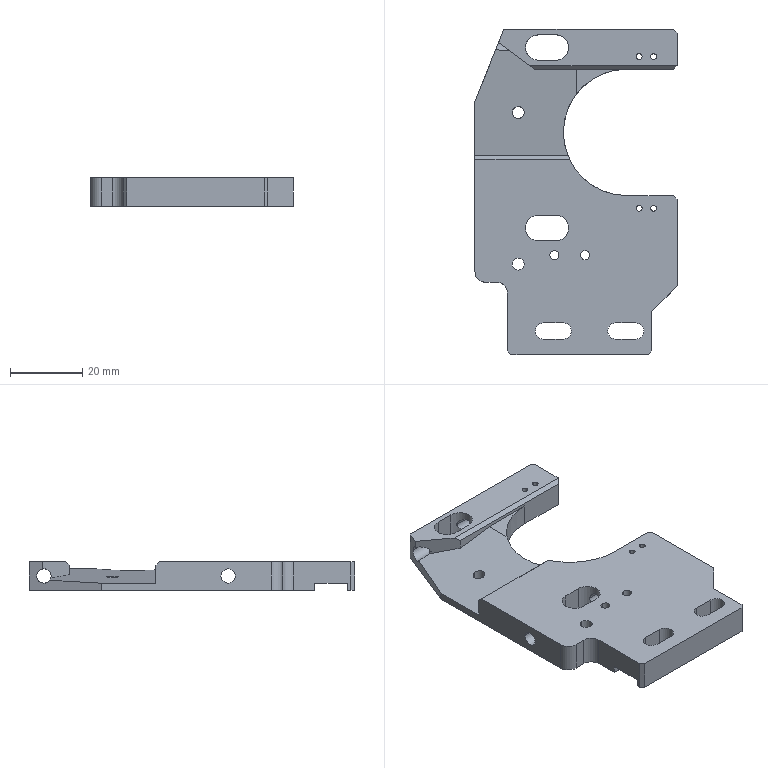NC program | NX | posted with a generic post | part box 56 x 90 x 8 mm
Whole program, first 1388 of 1533 lines:
N10 G17 G21 G94 G90
(ZLEVEL_PROFILE , TOOL : D10JING)
N12 T14 M6
N14 G54
N16 G17 G0 G90 X51.809 Y28.622 S7500 M3
N18 G43 Z30. H14
N20 Z-7.
N22 G94 G1 Z-8. F1000.
N24 X50.5 Y27.866
N26 G3 X50. Y27. R1.
N28 G1 Y-20.
N30 G2 X46.857 Y-24.642 R5.
N32 G1 X26.857 Y-32.642
N34 G2 X25. Y-33. R5.
N36 G1 X-22.
N38 G2 X-30. Y-25. R8.
N40 G1 Y-24.
N42 X-44.
N44 G2 X-47.536 Y-22.536 R5.
N46 G1 X-48.536 Y-21.536
N48 G2 X-50. Y-18. R5.
N50 G1 Y20.
N52 G2 X-48.536 Y23.536 R5.
N54 G1 X-47.536 Y24.536
N56 G2 X-44. Y26. R5.
N58 G1 X-35.071
N60 X-29.536 Y31.536
N62 G2 X-26. Y33. R5.
N64 G1 X-2.
N66 G2 X1.536 Y31.536 R5.
N68 G1 X2.536 Y30.536
N70 G2 X4. Y27. R5.
N72 G1 Y14.
N74 G3 X16.5 Y1.5 R12.5
N76 X29. Y14. R12.5
N78 G1 Y27.
N80 G2 X30.464 Y30.536 R5.
N82 G1 X31.464 Y31.536
N84 G2 X35. Y33. R5.
N86 G1 X44.
N88 G2 X47.536 Y31.536 R5.
N90 G1 X48.536 Y30.536
N92 G2 X50. Y27. R5.
N94 G3 X50.5 Y26.134 R1.
N96 G1 X52. Y25.268
N98 Z-7.
N100 G0 Z30.
N102 M5
(ZLEVEL_PROFILE_1 , TOOL : D4)
N104 T17 M6
N106 G54
N108 G17 G0 G90 X-8.5 Y-7.694 S7500 M3
N110 G43 Z30. H17
N112 Z1.5
N114 G94 G1 Y-5.199 Z1.369 F1000.
N116 X-8.75 Y-4.617 Z1.336
N118 X-9.214 Y-4.187 Z1.303
N120 X-9.782 Y-3.986 Z1.271
N122 X-10.542 Y-4.069 Z1.231
N124 X-11.167 Y-4.51 Z1.191
N126 X-11.5 Y-5.199 Z1.151
N128 Y-10.801 Z0.857
N130 X-11.17 Y-11.486 Z0.818
N132 X-10.55 Y-11.928 Z0.778
N134 X-9.795 Y-12.016 Z0.738
N136 X-9.225 Y-11.819 Z0.706
N138 X-8.754 Y-11.388 Z0.673
N140 X-8.5 Y-10.801 Z0.639
N142 Y-5.199 Z0.346
N144 X-8.75 Y-4.617 Z0.313
N146 X-9.214 Y-4.187 Z0.279
N148 X-9.782 Y-3.986 Z0.248
N150 X-10.542 Y-4.069 Z0.208
N152 X-11.167 Y-4.51 Z0.168
N154 X-11.5 Y-5.199 Z0.128
N156 Y-10.801 Z-0.166
N158 X-11.17 Y-11.486 Z-0.206
N160 X-10.55 Y-11.928 Z-0.246
N162 X-9.795 Y-12.016 Z-0.286
N164 X-9.225 Y-11.819 Z-0.317
N166 X-8.754 Y-11.388 Z-0.351
N168 X-8.5 Y-10.801 Z-0.384
N170 Y-10.5 Z-0.4
N172 Y-5.5 F1500.
N174 G3 X-10. Y-4. R1.5
N176 X-11.5 Y-5.5 R1.5
N178 G1 Y-10.5
N180 G3 X-10. Y-12. R1.5
N182 X-8.5 Y-10.5 R1.5
N184 G1 Y-5.644 Z-0.533
N186 X-8.539 Y-5.161 Z-0.547
N188 X-8.722 Y-4.714 Z-0.56
N190 X-8.899 Y-4.481 Z-0.568
N192 X-9.057 Y-4.37 Z-0.573
N194 X-9.375 Y-4.165 Z-0.584
N196 X-9.465 Y-4.129 Z-0.587
N198 X-9.773 Y-4.045 Z-0.596
N200 X-9.929 Y-4.024 Z-0.6
N202 X-10.209 Y-4.044 Z-0.608
N204 X-10.403 Y-4.075 Z-0.613
N206 X-10.63 Y-4.167 Z-0.62
N208 X-10.832 Y-4.283 Z-0.627
N210 X-11.045 Y-4.446 Z-0.634
N212 X-11.088 Y-4.501 Z-0.636
N214 X-11.174 Y-4.612 Z-0.64
N216 X-11.336 Y-4.881 Z-0.649
N218 X-11.399 Y-5.031 Z-0.653
N220 X-11.447 Y-5.213 Z-0.659
N222 X-11.483 Y-5.5 Z-0.667
N224 X-11.5 Y-5.743 Z-0.673
N226 Y-10.356 Z-0.8
N228 Y-10.5
N230 G3 X-10. Y-12. R1.5
N232 X-8.5 Y-10.5 R1.5
N234 G1 Y-5.644 Z-0.933
N236 X-8.539 Y-5.161 Z-0.947
N238 X-8.722 Y-4.714 Z-0.96
N240 X-8.899 Y-4.481 Z-0.968
N242 X-9.057 Y-4.37 Z-0.973
N244 X-9.375 Y-4.165 Z-0.984
N246 X-9.465 Y-4.129 Z-0.987
N248 X-9.773 Y-4.045 Z-0.996
N250 X-9.929 Y-4.024 Z-1.
N252 X-10.209 Y-4.044 Z-1.008
N254 X-10.403 Y-4.075 Z-1.013
N256 X-10.63 Y-4.167 Z-1.02
N258 X-10.832 Y-4.283 Z-1.027
N260 X-11.045 Y-4.446 Z-1.034
N262 X-11.088 Y-4.501 Z-1.036
N264 X-11.174 Y-4.612 Z-1.04
N266 X-11.336 Y-4.881 Z-1.049
N268 X-11.399 Y-5.031 Z-1.053
N270 X-11.447 Y-5.213 Z-1.059
N272 X-11.483 Y-5.5 Z-1.067
N274 X-11.5 Y-5.743 Z-1.073
N276 Y-10.356 Z-1.2
N278 Y-10.5
N280 G3 X-10. Y-12. R1.5
N282 X-8.5 Y-10.5 R1.5
N284 G1 Y-5.644 Z-1.333
N286 X-8.539 Y-5.161 Z-1.347
N288 X-8.722 Y-4.714 Z-1.36
N290 X-8.899 Y-4.481 Z-1.368
N292 X-9.057 Y-4.37 Z-1.373
N294 X-9.375 Y-4.165 Z-1.384
N296 X-9.465 Y-4.129 Z-1.387
N298 X-9.773 Y-4.045 Z-1.396
N300 X-9.929 Y-4.024 Z-1.4
N302 X-10.209 Y-4.044 Z-1.408
N304 X-10.403 Y-4.075 Z-1.413
N306 X-10.63 Y-4.167 Z-1.42
N308 X-10.832 Y-4.283 Z-1.427
N310 X-11.045 Y-4.446 Z-1.434
N312 X-11.088 Y-4.501 Z-1.436
N314 X-11.174 Y-4.612 Z-1.44
N316 X-11.336 Y-4.881 Z-1.449
N318 X-11.399 Y-5.031 Z-1.453
N320 X-11.447 Y-5.213 Z-1.459
N322 X-11.483 Y-5.5 Z-1.467
N324 X-11.5 Y-5.743 Z-1.473
N326 Y-10.356 Z-1.6
N328 Y-10.5
N330 G3 X-10. Y-12. R1.5
N332 X-8.5 Y-10.5 R1.5
N334 G1 Y-5.644 Z-1.733
N336 X-8.539 Y-5.161 Z-1.747
N338 X-8.722 Y-4.714 Z-1.76
N340 X-8.899 Y-4.481 Z-1.768
N342 X-9.057 Y-4.37 Z-1.773
N344 X-9.375 Y-4.165 Z-1.784
N346 X-9.465 Y-4.129 Z-1.787
N348 X-9.773 Y-4.045 Z-1.796
N350 X-9.929 Y-4.024 Z-1.8
N352 X-10.209 Y-4.044 Z-1.808
N354 X-10.403 Y-4.075 Z-1.813
N356 X-10.63 Y-4.167 Z-1.82
N358 X-10.832 Y-4.283 Z-1.827
N360 X-11.045 Y-4.446 Z-1.834
N362 X-11.088 Y-4.501 Z-1.836
N364 X-11.174 Y-4.612 Z-1.84
N366 X-11.336 Y-4.881 Z-1.849
N368 X-11.399 Y-5.031 Z-1.853
N370 X-11.447 Y-5.212 Z-1.859
N372 X-11.483 Y-5.5 Z-1.867
N374 X-11.5 Y-5.743 Z-1.873
N376 Y-10.356 Z-2.
N378 Y-10.5
N380 G3 X-10. Y-12. R1.5
N382 X-8.5 Y-10.5 R1.5
N384 G1 Y-5.644 Z-2.133
N386 X-8.539 Y-5.161 Z-2.147
N388 X-8.722 Y-4.714 Z-2.16
N390 X-8.899 Y-4.481 Z-2.168
N392 X-9.057 Y-4.37 Z-2.173
N394 X-9.375 Y-4.165 Z-2.184
N396 X-9.465 Y-4.129 Z-2.187
N398 X-9.773 Y-4.045 Z-2.196
N400 X-9.929 Y-4.024 Z-2.2
N402 X-10.209 Y-4.044 Z-2.208
N404 X-10.403 Y-4.075 Z-2.213
N406 X-10.63 Y-4.167 Z-2.22
N408 X-10.832 Y-4.283 Z-2.227
N410 X-11.045 Y-4.446 Z-2.234
N412 X-11.088 Y-4.501 Z-2.236
N414 X-11.174 Y-4.612 Z-2.24
N416 X-11.336 Y-4.88 Z-2.249
N418 X-11.399 Y-5.031 Z-2.253
N420 X-11.447 Y-5.212 Z-2.259
N422 X-11.483 Y-5.5 Z-2.267
N424 X-11.5 Y-5.743 Z-2.273
N426 Y-10.356 Z-2.4
N428 Y-10.5
N430 G3 X-10. Y-12. R1.5
N432 X-8.5 Y-10.5 R1.5
N434 G1 Y-5.644 Z-2.533
N436 X-8.539 Y-5.161 Z-2.547
N438 X-8.722 Y-4.714 Z-2.56
N440 X-8.899 Y-4.481 Z-2.568
N442 X-9.057 Y-4.37 Z-2.573
N444 X-9.375 Y-4.165 Z-2.584
N446 X-9.465 Y-4.129 Z-2.587
N448 X-9.773 Y-4.045 Z-2.596
N450 X-9.929 Y-4.024 Z-2.6
N452 X-10.209 Y-4.044 Z-2.608
N454 X-10.403 Y-4.075 Z-2.613
N456 X-10.63 Y-4.167 Z-2.62
N458 X-10.832 Y-4.283 Z-2.627
N460 X-11.045 Y-4.446 Z-2.634
N462 X-11.088 Y-4.501 Z-2.636
N464 X-11.174 Y-4.612 Z-2.64
N466 X-11.336 Y-4.88 Z-2.649
N468 X-11.399 Y-5.031 Z-2.653
N470 X-11.447 Y-5.212 Z-2.659
N472 X-11.483 Y-5.5 Z-2.667
N474 X-11.5 Y-5.743 Z-2.673
N476 Y-10.356 Z-2.8
N478 Y-10.5
N480 G3 X-10. Y-12. R1.5
N482 X-8.5 Y-10.5 R1.5
N484 G1 Y-5.644 Z-2.933
N486 X-8.539 Y-5.161 Z-2.947
N488 X-8.722 Y-4.714 Z-2.96
N490 X-8.899 Y-4.481 Z-2.968
N492 X-9.057 Y-4.37 Z-2.973
N494 X-9.375 Y-4.165 Z-2.984
N496 X-9.465 Y-4.129 Z-2.987
N498 X-9.773 Y-4.045 Z-2.996
N500 X-9.929 Y-4.024 Z-3.
N502 X-10.209 Y-4.044 Z-3.008
N504 X-10.403 Y-4.075 Z-3.013
N506 X-10.63 Y-4.167 Z-3.02
N508 X-10.832 Y-4.283 Z-3.027
N510 X-11.045 Y-4.446 Z-3.034
N512 X-11.088 Y-4.501 Z-3.036
N514 X-11.174 Y-4.612 Z-3.04
N516 X-11.336 Y-4.88 Z-3.049
N518 X-11.399 Y-5.031 Z-3.053
N520 X-11.447 Y-5.212 Z-3.059
N522 X-11.483 Y-5.5 Z-3.067
N524 X-11.5 Y-5.743 Z-3.073
N526 Y-10.356 Z-3.2
N528 Y-10.5
N530 G3 X-10. Y-12. R1.5
N532 X-8.5 Y-10.5 R1.5
N534 G1 Y-5.644 Z-3.333
N536 X-8.539 Y-5.161 Z-3.347
N538 X-8.722 Y-4.714 Z-3.36
N540 X-8.899 Y-4.481 Z-3.368
N542 X-9.057 Y-4.37 Z-3.373
N544 X-9.375 Y-4.165 Z-3.384
N546 X-9.465 Y-4.129 Z-3.387
N548 X-9.773 Y-4.046 Z-3.396
N550 X-9.929 Y-4.024 Z-3.4
N552 X-10.209 Y-4.044 Z-3.408
N554 X-10.403 Y-4.075 Z-3.413
N556 X-10.63 Y-4.167 Z-3.42
N558 X-10.832 Y-4.283 Z-3.427
N560 X-11.045 Y-4.446 Z-3.434
N562 X-11.088 Y-4.501 Z-3.436
N564 X-11.174 Y-4.612 Z-3.44
N566 X-11.336 Y-4.88 Z-3.449
N568 X-11.399 Y-5.031 Z-3.453
N570 X-11.447 Y-5.212 Z-3.459
N572 X-11.483 Y-5.5 Z-3.467
N574 X-11.5 Y-5.743 Z-3.473
N576 Y-10.356 Z-3.6
N578 Y-10.5
N580 G3 X-10. Y-12. R1.5
N582 X-8.5 Y-10.5 R1.5
N584 G1 Y-5.644 Z-3.733
N586 X-8.539 Y-5.161 Z-3.747
N588 X-8.722 Y-4.714 Z-3.76
N590 X-8.899 Y-4.481 Z-3.768
N592 X-9.057 Y-4.37 Z-3.773
N594 X-9.375 Y-4.165 Z-3.784
N596 X-9.465 Y-4.129 Z-3.787
N598 X-9.773 Y-4.046 Z-3.796
N600 X-9.929 Y-4.024 Z-3.8
N602 X-10.209 Y-4.044 Z-3.808
N604 X-10.403 Y-4.075 Z-3.813
N606 X-10.63 Y-4.167 Z-3.82
N608 X-10.832 Y-4.283 Z-3.827
N610 X-11.045 Y-4.446 Z-3.834
N612 X-11.088 Y-4.501 Z-3.836
N614 X-11.174 Y-4.612 Z-3.84
N616 X-11.336 Y-4.88 Z-3.849
N618 X-11.399 Y-5.031 Z-3.853
N620 X-11.447 Y-5.212 Z-3.859
N622 X-11.483 Y-5.5 Z-3.867
N624 X-11.5 Y-5.743 Z-3.873
N626 Y-10.356 Z-4.
N628 Y-10.5
N630 G3 X-10. Y-12. R1.5
N632 X-8.5 Y-10.5 R1.5
N634 G1 Y-5.644 Z-4.133
N636 X-8.539 Y-5.161 Z-4.147
N638 X-8.722 Y-4.714 Z-4.16
N640 X-8.899 Y-4.481 Z-4.168
N642 X-9.057 Y-4.37 Z-4.173
N644 X-9.375 Y-4.165 Z-4.184
N646 X-9.465 Y-4.129 Z-4.187
N648 X-9.773 Y-4.046 Z-4.196
N650 X-9.929 Y-4.024 Z-4.2
N652 X-10.209 Y-4.044 Z-4.208
N654 X-10.403 Y-4.075 Z-4.213
N656 X-10.629 Y-4.167 Z-4.22
N658 X-10.832 Y-4.283 Z-4.227
N660 X-11.045 Y-4.446 Z-4.234
N662 X-11.088 Y-4.501 Z-4.236
N664 X-11.174 Y-4.612 Z-4.24
N666 X-11.336 Y-4.88 Z-4.249
N668 X-11.399 Y-5.031 Z-4.253
N670 X-11.447 Y-5.212 Z-4.259
N672 X-11.483 Y-5.5 Z-4.267
N674 X-11.5 Y-5.743 Z-4.273
N676 Y-10.356 Z-4.4
N678 Y-10.5
N680 G3 X-10. Y-12. R1.5
N682 X-8.5 Y-10.5 R1.5
N684 G1 Y-5.644 Z-4.533
N686 X-8.539 Y-5.161 Z-4.547
N688 X-8.722 Y-4.714 Z-4.56
N690 X-8.899 Y-4.481 Z-4.568
N692 X-9.057 Y-4.37 Z-4.573
N694 X-9.375 Y-4.165 Z-4.584
N696 X-9.465 Y-4.129 Z-4.587
N698 X-9.773 Y-4.046 Z-4.596
N700 X-9.929 Y-4.024 Z-4.6
N702 X-10.209 Y-4.044 Z-4.608
N704 X-10.403 Y-4.075 Z-4.613
N706 X-10.629 Y-4.167 Z-4.62
N708 X-10.832 Y-4.283 Z-4.627
N710 X-11.045 Y-4.446 Z-4.634
N712 X-11.088 Y-4.501 Z-4.636
N714 X-11.174 Y-4.612 Z-4.64
N716 X-11.336 Y-4.88 Z-4.649
N718 X-11.399 Y-5.031 Z-4.653
N720 X-11.447 Y-5.212 Z-4.659
N722 X-11.483 Y-5.5 Z-4.667
N724 X-11.5 Y-5.743 Z-4.673
N726 Y-10.356 Z-4.8
N728 Y-10.5
N730 G3 X-10. Y-12. R1.5
N732 X-8.5 Y-10.5 R1.5
N734 G1 Y-5.644 Z-4.933
N736 X-8.539 Y-5.161 Z-4.947
N738 X-8.722 Y-4.714 Z-4.96
N740 X-8.899 Y-4.481 Z-4.968
N742 X-9.057 Y-4.37 Z-4.973
N744 X-9.375 Y-4.165 Z-4.984
N746 X-9.465 Y-4.129 Z-4.987
N748 X-9.773 Y-4.046 Z-4.996
N750 X-9.929 Y-4.024 Z-5.
N752 X-10.209 Y-4.044 Z-5.008
N754 X-10.403 Y-4.075 Z-5.013
N756 X-10.629 Y-4.167 Z-5.02
N758 X-10.832 Y-4.283 Z-5.027
N760 X-11.045 Y-4.446 Z-5.034
N762 X-11.088 Y-4.501 Z-5.036
N764 X-11.174 Y-4.612 Z-5.04
N766 X-11.335 Y-4.88 Z-5.049
N768 X-11.399 Y-5.031 Z-5.053
N770 X-11.447 Y-5.212 Z-5.059
N772 X-11.483 Y-5.5 Z-5.067
N774 X-11.5 Y-5.743 Z-5.073
N776 Y-10.356 Z-5.2
N778 Y-10.5
N780 G3 X-10. Y-12. R1.5
N782 X-8.5 Y-10.5 R1.5
N784 G1 Y-5.644 Z-5.333
N786 X-8.539 Y-5.161 Z-5.347
N788 X-8.722 Y-4.714 Z-5.36
N790 X-8.899 Y-4.481 Z-5.368
N792 X-9.057 Y-4.37 Z-5.373
N794 X-9.375 Y-4.165 Z-5.384
N796 X-9.465 Y-4.129 Z-5.387
N798 X-9.773 Y-4.046 Z-5.396
N800 X-9.929 Y-4.024 Z-5.4
N802 X-10.209 Y-4.044 Z-5.408
N804 X-10.403 Y-4.075 Z-5.413
N806 X-10.629 Y-4.167 Z-5.42
N808 X-10.832 Y-4.283 Z-5.427
N810 X-11.045 Y-4.446 Z-5.434
N812 X-11.088 Y-4.501 Z-5.436
N814 X-11.174 Y-4.612 Z-5.44
N816 X-11.335 Y-4.88 Z-5.449
N818 X-11.399 Y-5.031 Z-5.453
N820 X-11.447 Y-5.212 Z-5.459
N822 X-11.483 Y-5.5 Z-5.467
N824 X-11.5 Y-5.743 Z-5.473
N826 Y-10.356 Z-5.6
N828 Y-10.5
N830 G3 X-10. Y-12. R1.5
N832 X-8.5 Y-10.5 R1.5
N834 G1 Y-5.644 Z-5.733
N836 X-8.539 Y-5.161 Z-5.747
N838 X-8.722 Y-4.714 Z-5.76
N840 X-8.899 Y-4.481 Z-5.768
N842 X-9.057 Y-4.37 Z-5.773
N844 X-9.375 Y-4.165 Z-5.784
N846 X-9.465 Y-4.129 Z-5.787
N848 X-9.773 Y-4.046 Z-5.796
N850 X-9.929 Y-4.024 Z-5.8
N852 X-10.209 Y-4.044 Z-5.808
N854 X-10.403 Y-4.075 Z-5.813
N856 X-10.629 Y-4.167 Z-5.82
N858 X-10.832 Y-4.283 Z-5.827
N860 X-11.045 Y-4.446 Z-5.834
N862 X-11.088 Y-4.501 Z-5.836
N864 X-11.174 Y-4.612 Z-5.84
N866 X-11.335 Y-4.88 Z-5.849
N868 X-11.399 Y-5.031 Z-5.853
N870 X-11.447 Y-5.212 Z-5.859
N872 X-11.483 Y-5.5 Z-5.867
N874 X-11.5 Y-5.743 Z-5.873
N876 Y-10.356 Z-6.
N878 Y-10.5
N880 G3 X-10. Y-12. R1.5
N882 X-8.5 Y-10.5 R1.5
N884 G1 Y-5.644 Z-6.133
N886 X-8.539 Y-5.161 Z-6.147
N888 X-8.722 Y-4.714 Z-6.16
N890 X-8.899 Y-4.481 Z-6.168
N892 X-9.057 Y-4.37 Z-6.173
N894 X-9.375 Y-4.165 Z-6.184
N896 X-9.465 Y-4.129 Z-6.187
N898 X-9.773 Y-4.046 Z-6.196
N900 X-9.929 Y-4.024 Z-6.2
N902 X-10.209 Y-4.044 Z-6.208
N904 X-10.403 Y-4.075 Z-6.213
N906 X-10.629 Y-4.167 Z-6.22
N908 X-10.832 Y-4.283 Z-6.227
N910 X-11.045 Y-4.446 Z-6.234
N912 X-11.088 Y-4.501 Z-6.236
N914 X-11.174 Y-4.612 Z-6.24
N916 X-11.335 Y-4.88 Z-6.249
N918 X-11.399 Y-5.031 Z-6.253
N920 X-11.447 Y-5.212 Z-6.259
N922 X-11.483 Y-5.5 Z-6.267
N924 X-11.5 Y-5.743 Z-6.273
N926 Y-10.356 Z-6.4
N928 Y-10.5
N930 G3 X-10. Y-12. R1.5
N932 X-8.5 Y-10.5 R1.5
N934 G1 Y-5.644 Z-6.533
N936 X-8.539 Y-5.161 Z-6.547
N938 X-8.722 Y-4.714 Z-6.56
N940 X-8.899 Y-4.481 Z-6.568
N942 X-9.057 Y-4.37 Z-6.573
N944 X-9.375 Y-4.165 Z-6.584
N946 X-9.465 Y-4.129 Z-6.587
N948 X-9.773 Y-4.046 Z-6.596
N950 X-9.929 Y-4.024 Z-6.6
N952 X-10.209 Y-4.044 Z-6.608
N954 X-10.403 Y-4.075 Z-6.613
N956 X-10.629 Y-4.167 Z-6.62
N958 X-10.832 Y-4.283 Z-6.627
N960 X-11.045 Y-4.446 Z-6.634
N962 X-11.088 Y-4.501 Z-6.636
N964 X-11.174 Y-4.612 Z-6.64
N966 X-11.335 Y-4.88 Z-6.649
N968 X-11.399 Y-5.031 Z-6.653
N970 X-11.447 Y-5.212 Z-6.659
N972 X-11.483 Y-5.5 Z-6.667
N974 X-11.5 Y-5.743 Z-6.673
N976 Y-10.356 Z-6.8
N978 Y-10.5
N980 G3 X-10. Y-12. R1.5
N982 X-8.5 Y-10.5 R1.5
N984 G1 Y-5.644 Z-6.933
N986 X-8.539 Y-5.161 Z-6.947
N988 X-8.722 Y-4.714 Z-6.96
N990 X-8.899 Y-4.481 Z-6.968
N992 X-9.057 Y-4.37 Z-6.973
N994 X-9.375 Y-4.165 Z-6.984
N996 X-9.465 Y-4.129 Z-6.987
N998 X-9.773 Y-4.046 Z-6.996
N1000 X-9.929 Y-4.024 Z-7.
N1002 X-10.209 Y-4.044 Z-7.008
N1004 X-10.403 Y-4.075 Z-7.013
N1006 X-10.629 Y-4.167 Z-7.02
N1008 X-10.832 Y-4.283 Z-7.027
N1010 X-11.045 Y-4.446 Z-7.034
N1012 X-11.088 Y-4.501 Z-7.036
N1014 X-11.174 Y-4.612 Z-7.04
N1016 X-11.335 Y-4.88 Z-7.049
N1018 X-11.399 Y-5.031 Z-7.053
N1020 X-11.447 Y-5.212 Z-7.059
N1022 X-11.483 Y-5.5 Z-7.067
N1024 X-11.5 Y-5.743 Z-7.073
N1026 Y-10.356 Z-7.2
N1028 Y-10.5
N1030 G3 X-10. Y-12. R1.5
N1032 X-8.5 Y-10.5 R1.5
N1034 G1 Y-5.644 Z-7.333
N1036 X-8.539 Y-5.161 Z-7.347
N1038 X-8.722 Y-4.714 Z-7.36
N1040 X-8.899 Y-4.481 Z-7.368
N1042 X-9.057 Y-4.37 Z-7.373
N1044 X-9.375 Y-4.165 Z-7.384
N1046 X-9.465 Y-4.129 Z-7.387
N1048 X-9.773 Y-4.046 Z-7.396
N1050 X-9.929 Y-4.024 Z-7.4
N1052 X-10.209 Y-4.044 Z-7.408
N1054 X-10.403 Y-4.075 Z-7.413
N1056 X-10.629 Y-4.168 Z-7.42
N1058 X-10.832 Y-4.283 Z-7.427
N1060 X-11.045 Y-4.446 Z-7.434
N1062 X-11.088 Y-4.501 Z-7.436
N1064 X-11.174 Y-4.612 Z-7.44
N1066 X-11.335 Y-4.88 Z-7.449
N1068 X-11.399 Y-5.031 Z-7.453
N1070 X-11.447 Y-5.212 Z-7.459
N1072 X-11.483 Y-5.5 Z-7.467
N1074 X-11.5 Y-5.743 Z-7.473
N1076 Y-10.356 Z-7.6
N1078 Y-10.5
N1080 G3 X-10. Y-12. R1.5
N1082 X-8.5 Y-10.5 R1.5
N1084 G1 Y-5.644 Z-7.733
N1086 X-8.539 Y-5.161 Z-7.747
N1088 X-8.722 Y-4.714 Z-7.76
N1090 X-8.899 Y-4.481 Z-7.768
N1092 X-9.057 Y-4.37 Z-7.773
N1094 X-9.375 Y-4.165 Z-7.784
N1096 X-9.465 Y-4.129 Z-7.787
N1098 X-9.773 Y-4.046 Z-7.796
N1100 X-9.929 Y-4.024 Z-7.8
N1102 X-10.209 Y-4.044 Z-7.808
N1104 X-10.403 Y-4.075 Z-7.813
N1106 X-10.629 Y-4.168 Z-7.82
N1108 X-10.832 Y-4.283 Z-7.827
N1110 X-11.044 Y-4.446 Z-7.834
N1112 X-11.088 Y-4.501 Z-7.836
N1114 X-11.174 Y-4.612 Z-7.84
N1116 X-11.335 Y-4.88 Z-7.849
N1118 X-11.399 Y-5.031 Z-7.853
N1120 X-11.447 Y-5.212 Z-7.859
N1122 X-11.483 Y-5.5 Z-7.867
N1124 X-11.5 Y-5.743 Z-7.873
N1126 Y-10.356 Z-8.
N1128 Y-10.5
N1130 G3 X-10. Y-12. R1.5
N1132 X-8.5 Y-10.5 R1.5
N1134 G1 Y-5.5
N1136 G3 X-10. Y-4. R1.5
N1138 X-11.5 Y-5.5 R1.5
N1140 G1 Y-10.356
N1142 Z-6.5
N1144 G0 Z30.
N1146 X41.5 Y-7.694
N1148 Z1.5
N1150 G1 Y-5.199 Z1.369 F1000.
N1152 X41.25 Y-4.617 Z1.336
N1154 X40.786 Y-4.187 Z1.303
N1156 X40.218 Y-3.986 Z1.271
N1158 X39.458 Y-4.069 Z1.231
N1160 X38.833 Y-4.51 Z1.191
N1162 X38.5 Y-5.199 Z1.151
N1164 Y-10.801 Z0.857
N1166 X38.83 Y-11.486 Z0.818
N1168 X39.45 Y-11.928 Z0.778
N1170 X40.205 Y-12.016 Z0.738
N1172 X40.775 Y-11.819 Z0.706
N1174 X41.246 Y-11.388 Z0.673
N1176 X41.5 Y-10.801 Z0.639
N1178 Y-5.199 Z0.346
N1180 X41.25 Y-4.617 Z0.313
N1182 X40.786 Y-4.187 Z0.279
N1184 X40.218 Y-3.986 Z0.248
N1186 X39.458 Y-4.069 Z0.208
N1188 X38.833 Y-4.51 Z0.168
N1190 X38.5 Y-5.199 Z0.128
N1192 Y-10.801 Z-0.166
N1194 X38.83 Y-11.486 Z-0.206
N1196 X39.45 Y-11.928 Z-0.246
N1198 X40.205 Y-12.016 Z-0.286
N1200 X40.775 Y-11.819 Z-0.317
N1202 X41.246 Y-11.388 Z-0.351
N1204 X41.5 Y-10.801 Z-0.384
N1206 Y-10.5 Z-0.4
N1208 Y-5.5 F1500.
N1210 G3 X40. Y-4. R1.5
N1212 X38.5 Y-5.5 R1.5
N1214 G1 Y-10.5
N1216 G3 X40. Y-12. R1.5
N1218 X41.5 Y-10.5 R1.5
N1220 G1 Y-5.644 Z-0.533
N1222 X41.462 Y-5.323 Z-0.542
N1224 X41.439 Y-5.166 Z-0.547
N1226 X41.346 Y-4.904 Z-0.554
N1228 X41.26 Y-4.725 Z-0.56
N1230 X41.108 Y-4.528 Z-0.567
N1232 X40.943 Y-4.37 Z-0.573
N1234 X40.723 Y-4.206 Z-0.581
N1236 X40.535 Y-4.129 Z-0.587
N1238 X40.233 Y-4.047 Z-0.595
N1240 X40.071 Y-4.024 Z-0.6
N1242 X39.792 Y-4.044 Z-0.608
N1244 X39.597 Y-4.075 Z-0.613
N1246 X39.37 Y-4.167 Z-0.62
N1248 X39.168 Y-4.283 Z-0.627
N1250 X38.973 Y-4.434 Z-0.634
N1252 X38.826 Y-4.612 Z-0.64
N1254 X38.578 Y-5.023 Z-0.653
N1256 X38.5 Y-5.5 Z-0.667
N1258 Y-10.356 Z-0.8
N1260 Y-10.5
N1262 G3 X40. Y-12. R1.5
N1264 X41.5 Y-10.5 R1.5
N1266 G1 Y-5.644 Z-0.933
N1268 X41.462 Y-5.323 Z-0.942
N1270 X41.439 Y-5.166 Z-0.947
N1272 X41.346 Y-4.904 Z-0.954
N1274 X41.26 Y-4.725 Z-0.96
N1276 X41.108 Y-4.528 Z-0.967
N1278 X40.943 Y-4.37 Z-0.973
N1280 X40.723 Y-4.207 Z-0.981
N1282 X40.535 Y-4.129 Z-0.987
N1284 X40.233 Y-4.047 Z-0.995
N1286 X40.071 Y-4.024 Z-1.
N1288 X39.792 Y-4.044 Z-1.008
N1290 X39.597 Y-4.075 Z-1.013
N1292 X39.37 Y-4.167 Z-1.02
N1294 X39.168 Y-4.283 Z-1.027
N1296 X38.973 Y-4.434 Z-1.034
N1298 X38.826 Y-4.612 Z-1.04
N1300 X38.578 Y-5.023 Z-1.053
N1302 X38.5 Y-5.5 Z-1.067
N1304 Y-10.356 Z-1.2
N1306 Y-10.5
N1308 G3 X40. Y-12. R1.5
N1310 X41.5 Y-10.5 R1.5
N1312 G1 Y-5.644 Z-1.333
N1314 X41.462 Y-5.323 Z-1.342
N1316 X41.439 Y-5.166 Z-1.347
N1318 X41.346 Y-4.904 Z-1.354
N1320 X41.26 Y-4.725 Z-1.36
N1322 X41.108 Y-4.528 Z-1.367
N1324 X40.943 Y-4.37 Z-1.373
N1326 X40.723 Y-4.207 Z-1.381
N1328 X40.535 Y-4.129 Z-1.387
N1330 X40.233 Y-4.047 Z-1.395
N1332 X40.071 Y-4.024 Z-1.4
N1334 X39.792 Y-4.044 Z-1.408
N1336 X39.597 Y-4.075 Z-1.413
N1338 X39.37 Y-4.167 Z-1.42
N1340 X39.168 Y-4.283 Z-1.427
N1342 X38.973 Y-4.434 Z-1.434
N1344 X38.826 Y-4.612 Z-1.44
N1346 X38.578 Y-5.023 Z-1.453
N1348 X38.5 Y-5.5 Z-1.467
N1350 Y-10.356 Z-1.6
N1352 Y-10.5
N1354 G3 X40. Y-12. R1.5
N1356 X41.5 Y-10.5 R1.5
N1358 G1 Y-5.644 Z-1.733
N1360 X41.462 Y-5.323 Z-1.742
N1362 X41.439 Y-5.166 Z-1.747
N1364 X41.346 Y-4.904 Z-1.754
N1366 X41.26 Y-4.725 Z-1.76
N1368 X41.108 Y-4.529 Z-1.767
N1370 X40.943 Y-4.37 Z-1.773
N1372 X40.723 Y-4.207 Z-1.781
N1374 X40.535 Y-4.129 Z-1.787
N1376 X40.233 Y-4.047 Z-1.795
N1378 X40.071 Y-4.024 Z-1.8
N1380 X39.792 Y-4.044 Z-1.808
N1382 X39.597 Y-4.075 Z-1.813
N1384 X39.371 Y-4.167 Z-1.82
N1386 X39.168 Y-4.283 Z-1.827
N1388 X38.973 Y-4.434 Z-1.834
N1390 X38.826 Y-4.612 Z-1.84
N1392 X38.578 Y-5.023 Z-1.853
N1394 X38.5 Y-5.5 Z-1.867
N1396 Y-10.356 Z-2.
N1398 Y-10.5
N1400 G3 X40. Y-12. R1.5
N1402 X41.5 Y-10.5 R1.5
N1404 G1 Y-5.644 Z-2.133
N1406 X41.462 Y-5.323 Z-2.142
N1408 X41.439 Y-5.166 Z-2.147
N1410 X41.346 Y-4.904 Z-2.154
N1412 X41.26 Y-4.725 Z-2.16
N1414 X41.11 Y-4.527 Z-2.167
N1416 X40.943 Y-4.37 Z-2.173
N1418 X40.719 Y-4.204 Z-2.181
N1420 X40.535 Y-4.129 Z-2.187
N1422 X40.231 Y-4.046 Z-2.195
N1424 X40.071 Y-4.024 Z-2.2
N1426 X39.792 Y-4.044 Z-2.208
N1428 X39.597 Y-4.075 Z-2.213
N1430 X39.37 Y-4.167 Z-2.22
N1432 X39.168 Y-4.283 Z-2.227
N1434 X38.973 Y-4.434 Z-2.234
N1436 X38.826 Y-4.612 Z-2.24
N1438 X38.578 Y-5.023 Z-2.253
N1440 X38.5 Y-5.5 Z-2.267
N1442 Y-10.356 Z-2.4
N1444 Y-10.5
N1446 G3 X40. Y-12. R1.5
N1448 X41.5 Y-10.5 R1.5
N1450 G1 Y-5.644 Z-2.533
N1452 X41.462 Y-5.323 Z-2.542
N1454 X41.439 Y-5.166 Z-2.547
N1456 X41.346 Y-4.904 Z-2.554
N1458 X41.26 Y-4.725 Z-2.56
N1460 X41.11 Y-4.527 Z-2.567
N1462 X40.943 Y-4.37 Z-2.573
N1464 X40.719 Y-4.204 Z-2.581
N1466 X40.535 Y-4.129 Z-2.587
N1468 X40.231 Y-4.046 Z-2.595
N1470 X40.071 Y-4.024 Z-2.6
N1472 X39.792 Y-4.044 Z-2.608
N1474 X39.597 Y-4.075 Z-2.613
N1476 X39.371 Y-4.167 Z-2.62
N1478 X39.168 Y-4.283 Z-2.627
N1480 X38.973 Y-4.434 Z-2.634
N1482 X38.826 Y-4.612 Z-2.64
N1484 X38.578 Y-5.023 Z-2.653
N1486 X38.5 Y-5.5 Z-2.667
N1488 Y-10.356 Z-2.8
N1490 Y-10.5
N1492 G3 X40. Y-12. R1.5
N1494 X41.5 Y-10.5 R1.5
N1496 G1 Y-5.644 Z-2.933
N1498 X41.462 Y-5.323 Z-2.942
N1500 X41.439 Y-5.166 Z-2.947
N1502 X41.346 Y-4.904 Z-2.954
N1504 X41.26 Y-4.725 Z-2.96
N1506 X41.11 Y-4.527 Z-2.967
N1508 X40.943 Y-4.37 Z-2.973
N1510 X40.719 Y-4.205 Z-2.981
N1512 X40.535 Y-4.129 Z-2.987
N1514 X40.231 Y-4.046 Z-2.995
N1516 X40.071 Y-4.024 Z-3.
N1518 X39.792 Y-4.044 Z-3.008
N1520 X39.597 Y-4.075 Z-3.013
N1522 X39.371 Y-4.167 Z-3.02
N1524 X39.168 Y-4.283 Z-3.027
N1526 X38.973 Y-4.434 Z-3.034
N1528 X38.826 Y-4.612 Z-3.04
N1530 X38.578 Y-5.023 Z-3.053
N1532 X38.5 Y-5.5 Z-3.067
N1534 Y-10.356 Z-3.2
N1536 Y-10.5
N1538 G3 X40. Y-12. R1.5
N1540 X41.5 Y-10.5 R1.5
N1542 G1 Y-5.644 Z-3.333
N1544 X41.462 Y-5.323 Z-3.342
N1546 X41.439 Y-5.166 Z-3.347
N1548 X41.346 Y-4.904 Z-3.354
N1550 X41.26 Y-4.725 Z-3.36
N1552 X41.11 Y-4.527 Z-3.367
N1554 X40.943 Y-4.37 Z-3.373
N1556 X40.719 Y-4.205 Z-3.381
N1558 X40.535 Y-4.129 Z-3.387
N1560 X40.231 Y-4.046 Z-3.395
N1562 X40.071 Y-4.024 Z-3.4
N1564 X39.792 Y-4.044 Z-3.408
N1566 X39.597 Y-4.075 Z-3.413
N1568 X39.371 Y-4.167 Z-3.42
N1570 X39.168 Y-4.283 Z-3.427
N1572 X38.973 Y-4.434 Z-3.434
N1574 X38.826 Y-4.612 Z-3.44
N1576 X38.578 Y-5.023 Z-3.453
N1578 X38.5 Y-5.5 Z-3.467
N1580 Y-10.356 Z-3.6
N1582 Y-10.5
N1584 G3 X40. Y-12. R1.5
N1586 X41.5 Y-10.5 R1.5
N1588 G1 Y-5.644 Z-3.733
N1590 X41.462 Y-5.323 Z-3.742
N1592 X41.439 Y-5.166 Z-3.747
N1594 X41.346 Y-4.904 Z-3.754
N1596 X41.26 Y-4.725 Z-3.76
N1598 X41.11 Y-4.527 Z-3.767
N1600 X40.943 Y-4.37 Z-3.773
N1602 X40.719 Y-4.205 Z-3.781
N1604 X40.535 Y-4.129 Z-3.787
N1606 X40.231 Y-4.046 Z-3.795
N1608 X40.071 Y-4.024 Z-3.8
N1610 X39.792 Y-4.044 Z-3.808
N1612 X39.597 Y-4.075 Z-3.813
N1614 X39.371 Y-4.167 Z-3.82
N1616 X39.168 Y-4.283 Z-3.827
N1618 X38.973 Y-4.434 Z-3.834
N1620 X38.826 Y-4.612 Z-3.84
N1622 X38.578 Y-5.023 Z-3.853
N1624 X38.5 Y-5.5 Z-3.867
N1626 Y-10.356 Z-4.
N1628 Y-10.5
N1630 G3 X40. Y-12. R1.5
N1632 X41.5 Y-10.5 R1.5
N1634 G1 Y-5.644 Z-4.133
N1636 X41.462 Y-5.323 Z-4.142
N1638 X41.439 Y-5.166 Z-4.147
N1640 X41.346 Y-4.904 Z-4.154
N1642 X41.26 Y-4.725 Z-4.16
N1644 X41.11 Y-4.527 Z-4.167
N1646 X40.943 Y-4.37 Z-4.173
N1648 X40.719 Y-4.205 Z-4.181
N1650 X40.535 Y-4.129 Z-4.187
N1652 X40.231 Y-4.046 Z-4.195
N1654 X40.071 Y-4.024 Z-4.2
N1656 X39.792 Y-4.044 Z-4.208
N1658 X39.597 Y-4.075 Z-4.213
N1660 X39.371 Y-4.167 Z-4.22
N1662 X39.168 Y-4.283 Z-4.227
N1664 X38.973 Y-4.434 Z-4.234
N1666 X38.826 Y-4.612 Z-4.24
N1668 X38.578 Y-5.023 Z-4.253
N1670 X38.5 Y-5.5 Z-4.267
N1672 Y-10.356 Z-4.4
N1674 Y-10.5
N1676 G3 X40. Y-12. R1.5
N1678 X41.5 Y-10.5 R1.5
N1680 G1 Y-5.644 Z-4.533
N1682 X41.462 Y-5.323 Z-4.542
N1684 X41.439 Y-5.166 Z-4.547
N1686 X41.346 Y-4.904 Z-4.554
N1688 X41.26 Y-4.725 Z-4.56
N1690 X41.11 Y-4.527 Z-4.567
N1692 X40.943 Y-4.37 Z-4.573
N1694 X40.719 Y-4.205 Z-4.581
N1696 X40.535 Y-4.129 Z-4.587
N1698 X40.231 Y-4.047 Z-4.595
N1700 X40.071 Y-4.024 Z-4.6
N1702 X39.792 Y-4.044 Z-4.608
N1704 X39.597 Y-4.075 Z-4.613
N1706 X39.371 Y-4.167 Z-4.62
N1708 X39.168 Y-4.283 Z-4.627
N1710 X38.973 Y-4.434 Z-4.634
N1712 X38.826 Y-4.612 Z-4.64
N1714 X38.578 Y-5.023 Z-4.653
N1716 X38.5 Y-5.5 Z-4.667
N1718 Y-10.356 Z-4.8
N1720 Y-10.5
N1722 G3 X40. Y-12. R1.5
N1724 X41.5 Y-10.5 R1.5
N1726 G1 Y-5.644 Z-4.933
N1728 X41.462 Y-5.323 Z-4.942
N1730 X41.439 Y-5.166 Z-4.947
N1732 X41.346 Y-4.904 Z-4.954
N1734 X41.26 Y-4.725 Z-4.96
N1736 X41.11 Y-4.527 Z-4.967
N1738 X40.943 Y-4.37 Z-4.973
N1740 X40.719 Y-4.205 Z-4.981
N1742 X40.535 Y-4.129 Z-4.987
N1744 X40.231 Y-4.047 Z-4.995
N1746 X40.071 Y-4.024 Z-5.
N1748 X39.792 Y-4.044 Z-5.008
N1750 X39.597 Y-4.075 Z-5.013
N1752 X39.371 Y-4.167 Z-5.02
N1754 X39.168 Y-4.283 Z-5.027
N1756 X38.973 Y-4.434 Z-5.034
N1758 X38.826 Y-4.612 Z-5.04
N1760 X38.578 Y-5.023 Z-5.053
N1762 X38.5 Y-5.5 Z-5.067
N1764 Y-10.356 Z-5.2
N1766 Y-10.5
N1768 G3 X40. Y-12. R1.5
N1770 X41.5 Y-10.5 R1.5
N1772 G1 Y-5.644 Z-5.333
N1774 X41.462 Y-5.323 Z-5.342
N1776 X41.439 Y-5.166 Z-5.347
N1778 X41.346 Y-4.904 Z-5.354
N1780 X41.26 Y-4.725 Z-5.36
N1782 X41.11 Y-4.527 Z-5.367
N1784 X40.943 Y-4.37 Z-5.373
N1786 X40.719 Y-4.205 Z-5.381
N1788 X40.535 Y-4.129 Z-5.387
N1790 X40.231 Y-4.047 Z-5.395
N1792 X40.071 Y-4.024 Z-5.4
N1794 X39.792 Y-4.044 Z-5.408
N1796 X39.597 Y-4.075 Z-5.413
N1798 X39.371 Y-4.167 Z-5.42
N1800 X39.168 Y-4.283 Z-5.427
N1802 X38.973 Y-4.434 Z-5.434
N1804 X38.826 Y-4.612 Z-5.44
N1806 X38.578 Y-5.023 Z-5.453
N1808 X38.5 Y-5.5 Z-5.467
N1810 Y-10.356 Z-5.6
N1812 Y-10.5
N1814 G3 X40. Y-12. R1.5
N1816 X41.5 Y-10.5 R1.5
N1818 G1 Y-5.644 Z-5.733
N1820 X41.462 Y-5.323 Z-5.742
N1822 X41.439 Y-5.166 Z-5.747
N1824 X41.346 Y-4.904 Z-5.754
N1826 X41.26 Y-4.725 Z-5.76
N1828 X41.11 Y-4.527 Z-5.767
N1830 X40.943 Y-4.37 Z-5.773
N1832 X40.719 Y-4.205 Z-5.781
N1834 X40.535 Y-4.129 Z-5.787
N1836 X40.231 Y-4.047 Z-5.795
N1838 X40.071 Y-4.024 Z-5.8
N1840 X39.792 Y-4.044 Z-5.808
N1842 X39.597 Y-4.075 Z-5.813
N1844 X39.371 Y-4.167 Z-5.82
N1846 X39.168 Y-4.283 Z-5.827
N1848 X38.973 Y-4.434 Z-5.834
N1850 X38.826 Y-4.612 Z-5.84
N1852 X38.578 Y-5.023 Z-5.853
N1854 X38.5 Y-5.5 Z-5.867
N1856 Y-10.356 Z-6.
N1858 Y-10.5
N1860 G3 X40. Y-12. R1.5
N1862 X41.5 Y-10.5 R1.5
N1864 G1 Y-5.644 Z-6.133
N1866 X41.462 Y-5.323 Z-6.142
N1868 X41.439 Y-5.166 Z-6.147
N1870 X41.346 Y-4.904 Z-6.154
N1872 X41.26 Y-4.725 Z-6.16
N1874 X41.11 Y-4.527 Z-6.167
N1876 X40.943 Y-4.37 Z-6.173
N1878 X40.719 Y-4.205 Z-6.181
N1880 X40.535 Y-4.129 Z-6.187
N1882 X40.231 Y-4.047 Z-6.195
N1884 X40.071 Y-4.024 Z-6.2
N1886 X39.792 Y-4.044 Z-6.208
N1888 X39.597 Y-4.075 Z-6.213
N1890 X39.371 Y-4.167 Z-6.22
N1892 X39.168 Y-4.283 Z-6.227
N1894 X38.973 Y-4.434 Z-6.234
N1896 X38.826 Y-4.612 Z-6.24
N1898 X38.578 Y-5.023 Z-6.253
N1900 X38.5 Y-5.5 Z-6.267
N1902 Y-10.356 Z-6.4
N1904 Y-10.5
N1906 G3 X40. Y-12. R1.5
N1908 X41.5 Y-10.5 R1.5
N1910 G1 Y-5.644 Z-6.533
N1912 X41.462 Y-5.323 Z-6.542
N1914 X41.439 Y-5.166 Z-6.547
N1916 X41.346 Y-4.904 Z-6.554
N1918 X41.26 Y-4.725 Z-6.56
N1920 X41.11 Y-4.528 Z-6.567
N1922 X40.943 Y-4.37 Z-6.573
N1924 X40.719 Y-4.205 Z-6.581
N1926 X40.535 Y-4.129 Z-6.587
N1928 X40.231 Y-4.047 Z-6.595
N1930 X40.071 Y-4.024 Z-6.6
N1932 X39.792 Y-4.044 Z-6.608
N1934 X39.597 Y-4.075 Z-6.613
N1936 X39.371 Y-4.167 Z-6.62
N1938 X39.168 Y-4.283 Z-6.627
N1940 X38.973 Y-4.434 Z-6.634
N1942 X38.826 Y-4.612 Z-6.64
N1944 X38.578 Y-5.023 Z-6.653
N1946 X38.5 Y-5.5 Z-6.667
N1948 Y-10.356 Z-6.8
N1950 Y-10.5
N1952 G3 X40. Y-12. R1.5
N1954 X41.5 Y-10.5 R1.5
N1956 G1 Y-5.644 Z-6.933
N1958 X41.462 Y-5.323 Z-6.942
N1960 X41.439 Y-5.166 Z-6.947
N1962 X41.346 Y-4.904 Z-6.954
N1964 X41.26 Y-4.725 Z-6.96
N1966 X41.11 Y-4.528 Z-6.967
N1968 X40.943 Y-4.37 Z-6.973
N1970 X40.719 Y-4.205 Z-6.981
N1972 X40.535 Y-4.129 Z-6.987
N1974 X40.232 Y-4.047 Z-6.995
N1976 X40.071 Y-4.024 Z-7.
N1978 X39.792 Y-4.044 Z-7.008
N1980 X39.597 Y-4.075 Z-7.013
N1982 X39.371 Y-4.167 Z-7.02
N1984 X39.168 Y-4.283 Z-7.027
N1986 X38.973 Y-4.434 Z-7.034
N1988 X38.826 Y-4.612 Z-7.04
N1990 X38.578 Y-5.023 Z-7.053
N1992 X38.5 Y-5.5 Z-7.067
N1994 Y-10.356 Z-7.2
N1996 Y-10.5
N1998 G3 X40. Y-12. R1.5
N2000 X41.5 Y-10.5 R1.5
N2002 G1 Y-5.644 Z-7.333
N2004 X41.462 Y-5.323 Z-7.342
N2006 X41.439 Y-5.166 Z-7.347
N2008 X41.346 Y-4.904 Z-7.354
N2010 X41.26 Y-4.725 Z-7.36
N2012 X41.11 Y-4.528 Z-7.367
N2014 X40.943 Y-4.37 Z-7.373
N2016 X40.719 Y-4.205 Z-7.381
N2018 X40.535 Y-4.129 Z-7.387
N2020 X40.232 Y-4.047 Z-7.395
N2022 X40.071 Y-4.024 Z-7.4
N2024 X39.792 Y-4.044 Z-7.408
N2026 X39.597 Y-4.075 Z-7.413
N2028 X39.371 Y-4.167 Z-7.42
N2030 X39.168 Y-4.283 Z-7.427
N2032 X38.973 Y-4.434 Z-7.434
N2034 X38.826 Y-4.612 Z-7.44
N2036 X38.578 Y-5.023 Z-7.453
N2038 X38.5 Y-5.5 Z-7.467
N2040 Y-10.356 Z-7.6
N2042 Y-10.5
N2044 G3 X40. Y-12. R1.5
N2046 X41.5 Y-10.5 R1.5
N2048 G1 Y-5.644 Z-7.733
N2050 X41.462 Y-5.323 Z-7.742
N2052 X41.439 Y-5.166 Z-7.747
N2054 X41.346 Y-4.904 Z-7.754
N2056 X41.26 Y-4.725 Z-7.76
N2058 X41.11 Y-4.528 Z-7.767
N2060 X40.943 Y-4.37 Z-7.773
N2062 X40.719 Y-4.205 Z-7.781
N2064 X40.535 Y-4.129 Z-7.787
N2066 X40.232 Y-4.047 Z-7.795
N2068 X40.071 Y-4.024 Z-7.8
N2070 X39.792 Y-4.044 Z-7.808
N2072 X39.597 Y-4.075 Z-7.813
N2074 X39.371 Y-4.167 Z-7.82
N2076 X39.168 Y-4.283 Z-7.827
N2078 X38.973 Y-4.434 Z-7.834
N2080 X38.826 Y-4.612 Z-7.84
N2082 X38.578 Y-5.023 Z-7.853
N2084 X38.5 Y-5.5 Z-7.867
N2086 Y-10.356 Z-8.
N2088 Y-10.5
N2090 G3 X40. Y-12. R1.5
N2092 X41.5 Y-10.5 R1.5
N2094 G1 Y-5.5
N2096 G3 X40. Y-4. R1.5
N2098 X38.5 Y-5.5 R1.5
N2100 G1 Y-10.356
N2102 Z-6.5
N2104 G0 Z30.
(ZLEVEL_PROFILE_1_COPY , TOOL : D4)
N2106 X-38.25 Y-8.066
N2108 Z-0.5
N2110 G1 Y-3.588 Z-0.735 F1000.
N2112 X-38.258 Y-3.438 Z-0.743
N2114 X-38.289 Y-3.315 Z-0.749
N2116 X-38.502 Y-3.22 Z-0.761
N2118 X-38.702 Y-3.322 Z-0.773
N2120 X-38.735 Y-3.415 Z-0.778
N2122 X-38.75 Y-3.59 Z-0.788
N2124 Y-8.911 Z-1.066
N2126 X-38.745 Y-9.051 Z-1.074
N2128 X-38.733 Y-9.105 Z-1.077
N2130 X-38.625 Y-9.25 Z-1.086
N2132 X-38.374 Z-1.099
N2134 X-38.278 Y-9.121 Z-1.108
N2136 X-38.266 Y-9.089 Z-1.109
N2138 X-38.25 Y-8.908 Z-1.119
N2140 Y-3.588 Z-1.398
N2142 X-38.258 Y-3.438 Z-1.406
N2144 X-38.289 Y-3.315 Z-1.412
N2146 X-38.502 Y-3.22 Z-1.425
N2148 X-38.702 Y-3.322 Z-1.436
N2150 X-38.735 Y-3.415 Z-1.441
N2152 X-38.75 Y-3.59 Z-1.451
N2154 Y-8.911 Z-1.73
N2156 X-38.745 Y-9.051 Z-1.737
N2158 X-38.733 Y-9.105 Z-1.74
N2160 X-38.625 Y-9.25 Z-1.749
N2162 X-38.374 Z-1.762
N2164 X-38.278 Y-9.121 Z-1.771
N2166 X-38.266 Y-9.089 Z-1.773
N2168 X-38.25 Y-8.908 Z-1.782
N2170 Y-3.588 Z-2.061
N2172 X-38.258 Y-3.438 Z-2.069
N2174 X-38.289 Y-3.315 Z-2.075
N2176 X-38.502 Y-3.22 Z-2.088
N2178 X-38.702 Y-3.322 Z-2.099
N2180 X-38.735 Y-3.415 Z-2.105
N2182 X-38.75 Y-3.59 Z-2.114
N2184 Y-8.911 Z-2.393
N2186 X-38.745 Y-9.051 Z-2.4
N2188 G3 X-38.266 Y-9.089 R0.25 F1500.
N2190 G1 X-38.25 Y-8.908
N2192 Y-3.588
N2194 X-38.258 Y-3.438
N2196 G3 X-38.735 Y-3.415 R0.25
N2198 G1 X-38.75 Y-3.59
N2200 Y-8.911
N2202 X-38.745 Y-9.051
N2204 X-38.597 Y-9.23 Z-2.41
N2206 X-38.365 Y-9.211 Z-2.421
N2208 X-38.259 Y-9.007 Z-2.431
N2210 X-38.25 Y-8.766 Z-2.441
N2212 Y-3.69 Z-2.656
N2214 X-38.257 Y-3.449 Z-2.667
N2216 X-38.403 Y-3.269 Z-2.677
N2218 X-38.635 Y-3.289 Z-2.687
N2220 X-38.742 Y-3.493 Z-2.697
N2222 X-38.75 Y-3.734 Z-2.708
N2224 Y-5.909 Z-2.8
N2226 Y-8.911
N2228 X-38.745 Y-9.051
N2230 X-38.597 Y-9.23 Z-2.81
N2232 X-38.365 Y-9.211 Z-2.821
N2234 X-38.259 Y-9.007 Z-2.831
N2236 X-38.25 Y-8.766 Z-2.841
N2238 Y-3.69 Z-3.056
N2240 X-38.257 Y-3.449 Z-3.067
N2242 X-38.403 Y-3.269 Z-3.077
N2244 X-38.635 Y-3.289 Z-3.087
N2246 X-38.742 Y-3.493 Z-3.097
N2248 X-38.75 Y-3.734 Z-3.108
N2250 Y-5.909 Z-3.2
N2252 Y-8.911
N2254 X-38.745 Y-9.051
N2256 X-38.597 Y-9.23 Z-3.21
N2258 X-38.365 Y-9.211 Z-3.221
N2260 X-38.259 Y-9.007 Z-3.231
N2262 X-38.25 Y-8.766 Z-3.241
N2264 Y-3.69 Z-3.456
N2266 X-38.257 Y-3.449 Z-3.467
N2268 X-38.403 Y-3.269 Z-3.477
N2270 X-38.635 Y-3.289 Z-3.487
N2272 X-38.742 Y-3.493 Z-3.497
N2274 X-38.75 Y-3.734 Z-3.508
N2276 Y-5.909 Z-3.6
N2278 Y-8.911
N2280 X-38.745 Y-9.051
N2282 X-38.597 Y-9.23 Z-3.61
N2284 X-38.365 Y-9.211 Z-3.621
N2286 X-38.259 Y-9.007 Z-3.631
N2288 X-38.25 Y-8.766 Z-3.641
N2290 Y-3.69 Z-3.856
N2292 X-38.257 Y-3.449 Z-3.867
N2294 X-38.403 Y-3.269 Z-3.877
N2296 X-38.635 Y-3.289 Z-3.887
N2298 X-38.742 Y-3.493 Z-3.897
N2300 X-38.75 Y-3.734 Z-3.908
N2302 Y-5.909 Z-4.
N2304 Y-8.911
N2306 X-38.745 Y-9.051
N2308 X-38.597 Y-9.23 Z-4.01
N2310 X-38.365 Y-9.211 Z-4.021
N2312 X-38.259 Y-9.007 Z-4.031
N2314 X-38.25 Y-8.766 Z-4.041
N2316 Y-3.69 Z-4.256
N2318 X-38.257 Y-3.449 Z-4.267
N2320 X-38.403 Y-3.269 Z-4.277
N2322 X-38.635 Y-3.289 Z-4.287
N2324 X-38.742 Y-3.493 Z-4.297
N2326 X-38.75 Y-3.734 Z-4.308
N2328 Y-5.909 Z-4.4
N2330 Y-8.911
N2332 X-38.745 Y-9.051
N2334 X-38.597 Y-9.23 Z-4.41
N2336 X-38.365 Y-9.211 Z-4.421
N2338 X-38.259 Y-9.007 Z-4.431
N2340 X-38.25 Y-8.766 Z-4.441
N2342 Y-3.69 Z-4.656
N2344 X-38.257 Y-3.449 Z-4.667
N2346 X-38.403 Y-3.269 Z-4.677
N2348 X-38.635 Y-3.289 Z-4.687
N2350 X-38.742 Y-3.493 Z-4.697
N2352 X-38.75 Y-3.734 Z-4.708
N2354 Y-5.909 Z-4.8
N2356 Y-8.911
N2358 X-38.745 Y-9.051
N2360 X-38.597 Y-9.23 Z-4.81
N2362 X-38.365 Y-9.211 Z-4.821
N2364 X-38.259 Y-9.007 Z-4.831
N2366 X-38.25 Y-8.766 Z-4.841
N2368 Y-3.69 Z-5.056
N2370 X-38.257 Y-3.449 Z-5.067
N2372 X-38.403 Y-3.269 Z-5.077
N2374 X-38.635 Y-3.289 Z-5.087
N2376 X-38.742 Y-3.493 Z-5.097
N2378 X-38.75 Y-3.734 Z-5.108
N2380 Y-5.909 Z-5.2
N2382 Y-8.911
N2384 X-38.745 Y-9.051
N2386 X-38.597 Y-9.23 Z-5.21
N2388 X-38.365 Y-9.211 Z-5.221
N2390 X-38.259 Y-9.007 Z-5.231
N2392 X-38.25 Y-8.766 Z-5.241
N2394 Y-3.69 Z-5.456
N2396 X-38.257 Y-3.449 Z-5.467
N2398 X-38.403 Y-3.269 Z-5.477
N2400 X-38.635 Y-3.289 Z-5.487
N2402 X-38.742 Y-3.493 Z-5.497
N2404 X-38.75 Y-3.734 Z-5.508
N2406 Y-5.909 Z-5.6
N2408 Y-8.911
N2410 X-38.745 Y-9.051
N2412 X-38.597 Y-9.23 Z-5.61
N2414 X-38.365 Y-9.211 Z-5.621
N2416 X-38.259 Y-9.007 Z-5.631
N2418 X-38.25 Y-8.766 Z-5.641
N2420 Y-3.69 Z-5.856
N2422 X-38.257 Y-3.449 Z-5.867
N2424 X-38.403 Y-3.269 Z-5.877
N2426 X-38.635 Y-3.289 Z-5.887
N2428 X-38.742 Y-3.493 Z-5.897
N2430 X-38.75 Y-3.734 Z-5.908
N2432 Y-5.909 Z-6.
N2434 Y-8.911
N2436 X-38.745 Y-9.051
N2438 X-38.597 Y-9.23 Z-6.01
N2440 X-38.365 Y-9.211 Z-6.021
N2442 X-38.259 Y-9.007 Z-6.031
N2444 X-38.25 Y-8.766 Z-6.041
N2446 Y-3.69 Z-6.256
N2448 X-38.257 Y-3.449 Z-6.267
N2450 X-38.403 Y-3.269 Z-6.277
N2452 X-38.635 Y-3.289 Z-6.287
N2454 X-38.742 Y-3.493 Z-6.297
N2456 X-38.75 Y-3.734 Z-6.308
N2458 Y-5.909 Z-6.4
N2460 Y-8.911
N2462 X-38.745 Y-9.051
N2464 X-38.597 Y-9.23 Z-6.41
N2466 X-38.365 Y-9.211 Z-6.421
N2468 X-38.259 Y-9.007 Z-6.431
N2470 X-38.25 Y-8.766 Z-6.441
N2472 Y-3.69 Z-6.656
N2474 X-38.257 Y-3.449 Z-6.667
N2476 X-38.403 Y-3.269 Z-6.677
N2478 X-38.635 Y-3.289 Z-6.687
N2480 X-38.742 Y-3.493 Z-6.697
N2482 X-38.75 Y-3.734 Z-6.708
N2484 Y-5.909 Z-6.8
N2486 Y-8.911
N2488 X-38.745 Y-9.051
N2490 X-38.597 Y-9.23 Z-6.81
N2492 X-38.365 Y-9.211 Z-6.821
N2494 X-38.259 Y-9.007 Z-6.831
N2496 X-38.25 Y-8.766 Z-6.841
N2498 Y-3.69 Z-7.056
N2500 X-38.257 Y-3.449 Z-7.067
N2502 X-38.403 Y-3.269 Z-7.077
N2504 X-38.635 Y-3.289 Z-7.087
N2506 X-38.742 Y-3.493 Z-7.097
N2508 X-38.75 Y-3.734 Z-7.108
N2510 Y-5.909 Z-7.2
N2512 Y-8.911
N2514 X-38.745 Y-9.051
N2516 X-38.597 Y-9.23 Z-7.21
N2518 X-38.365 Y-9.211 Z-7.221
N2520 X-38.259 Y-9.007 Z-7.231
N2522 X-38.25 Y-8.766 Z-7.241
N2524 Y-3.69 Z-7.456
N2526 X-38.257 Y-3.449 Z-7.467
N2528 X-38.403 Y-3.269 Z-7.477
N2530 X-38.635 Y-3.289 Z-7.487
N2532 X-38.742 Y-3.493 Z-7.497
N2534 X-38.75 Y-3.734 Z-7.508
N2536 Y-5.909 Z-7.6
N2538 Y-8.911
N2540 X-38.745 Y-9.051
N2542 X-38.597 Y-9.23 Z-7.61
N2544 X-38.365 Y-9.211 Z-7.621
N2546 X-38.259 Y-9.007 Z-7.631
N2548 X-38.25 Y-8.766 Z-7.641
N2550 Y-3.69 Z-7.856
N2552 X-38.257 Y-3.449 Z-7.867
N2554 X-38.403 Y-3.269 Z-7.877
N2556 X-38.635 Y-3.289 Z-7.887
N2558 X-38.742 Y-3.493 Z-7.897
N2560 X-38.75 Y-3.734 Z-7.908
N2562 Y-5.909 Z-8.
N2564 Y-8.911
N2566 X-38.745 Y-9.051
N2568 G3 X-38.266 Y-9.089 R0.25
N2570 G1 X-38.25 Y-8.908
N2572 Y-3.588
N2574 X-38.258 Y-3.438
N2576 G3 X-38.735 Y-3.415 R0.25
N2578 G1 X-38.75 Y-3.59
N2580 Y-5.909
N2582 Z-6.5
N2584 G0 Z30.
N2586 Y15.566
N2588 Z-0.5
N2590 G1 Y11.088 Z-0.735 F1000.
N2592 X-38.742 Y10.938 Z-0.743
N2594 X-38.711 Y10.815 Z-0.749
N2596 X-38.498 Y10.72 Z-0.761
N2598 X-38.298 Y10.822 Z-0.773
N2600 X-38.265 Y10.915 Z-0.778
N2602 X-38.25 Y11.09 Z-0.788
N2604 Y16.411 Z-1.066
N2606 X-38.255 Y16.551 Z-1.074
N2608 X-38.267 Y16.605 Z-1.077
N2610 X-38.375 Y16.75 Z-1.086
N2612 X-38.626 Z-1.099
N2614 X-38.722 Y16.621 Z-1.108
N2616 X-38.734 Y16.589 Z-1.109
N2618 X-38.75 Y16.408 Z-1.119
N2620 Y11.088 Z-1.398
N2622 X-38.742 Y10.938 Z-1.406
N2624 X-38.711 Y10.815 Z-1.412
N2626 X-38.498 Y10.72 Z-1.425
N2628 X-38.298 Y10.822 Z-1.436
N2630 X-38.265 Y10.915 Z-1.441
N2632 X-38.25 Y11.09 Z-1.451
N2634 Y16.411 Z-1.73
N2636 X-38.255 Y16.551 Z-1.737
N2638 X-38.267 Y16.605 Z-1.74
N2640 X-38.375 Y16.75 Z-1.749
N2642 X-38.626 Z-1.762
N2644 X-38.722 Y16.621 Z-1.771
N2646 X-38.734 Y16.589 Z-1.773
N2648 X-38.75 Y16.408 Z-1.782
N2650 Y11.088 Z-2.061
N2652 X-38.742 Y10.938 Z-2.069
N2654 X-38.711 Y10.815 Z-2.075
N2656 X-38.498 Y10.72 Z-2.088
N2658 X-38.298 Y10.822 Z-2.099
N2660 X-38.265 Y10.915 Z-2.105
N2662 X-38.25 Y11.09 Z-2.114
N2664 Y16.411 Z-2.393
N2666 X-38.255 Y16.551 Z-2.4
N2668 G3 X-38.734 Y16.589 R0.25 F1500.
N2670 G1 X-38.75 Y16.408
N2672 Y11.088
N2674 X-38.742 Y10.938
N2676 G3 X-38.265 Y10.915 R0.25
N2678 G1 X-38.25 Y11.09
N2680 Y16.411
N2682 X-38.255 Y16.551
N2684 X-38.403 Y16.73 Z-2.41
N2686 X-38.635 Y16.711 Z-2.421
N2688 X-38.741 Y16.507 Z-2.431
N2690 X-38.75 Y16.266 Z-2.441
N2692 Y11.19 Z-2.656
N2694 X-38.743 Y10.949 Z-2.667
N2696 X-38.597 Y10.769 Z-2.677
N2698 X-38.365 Y10.789 Z-2.687
N2700 X-38.258 Y10.993 Z-2.697
N2702 X-38.25 Y11.234 Z-2.708
N2704 Y13.409 Z-2.8
N2706 Y16.411
N2708 X-38.255 Y16.551
N2710 X-38.403 Y16.73 Z-2.81
N2712 X-38.635 Y16.711 Z-2.821
N2714 X-38.741 Y16.507 Z-2.831
N2716 X-38.75 Y16.266 Z-2.841
N2718 Y11.19 Z-3.056
N2720 X-38.743 Y10.949 Z-3.067
N2722 X-38.597 Y10.769 Z-3.077
N2724 X-38.365 Y10.789 Z-3.087
N2726 X-38.258 Y10.993 Z-3.097
N2728 X-38.25 Y11.234 Z-3.108
N2730 Y13.409 Z-3.2
N2732 Y16.411
N2734 X-38.255 Y16.551
N2736 X-38.403 Y16.73 Z-3.21
N2738 X-38.635 Y16.711 Z-3.221
N2740 X-38.741 Y16.507 Z-3.231
N2742 X-38.75 Y16.266 Z-3.241
N2744 Y11.19 Z-3.456
N2746 X-38.743 Y10.949 Z-3.467
N2748 X-38.597 Y10.769 Z-3.477
N2750 X-38.365 Y10.789 Z-3.487
N2752 X-38.258 Y10.993 Z-3.497
N2754 X-38.25 Y11.234 Z-3.508
N2756 Y13.409 Z-3.6
N2758 Y16.411
N2760 X-38.255 Y16.551
N2762 X-38.403 Y16.73 Z-3.61
N2764 X-38.635 Y16.711 Z-3.621
N2766 X-38.741 Y16.507 Z-3.631
N2768 X-38.75 Y16.266 Z-3.641
N2770 Y11.19 Z-3.856
N2772 X-38.743 Y10.949 Z-3.867
N2774 X-38.597 Y10.769 Z-3.877
N2776 X-38.365 Y10.789 Z-3.887
N2778 X-38.258 Y10.993 Z-3.897